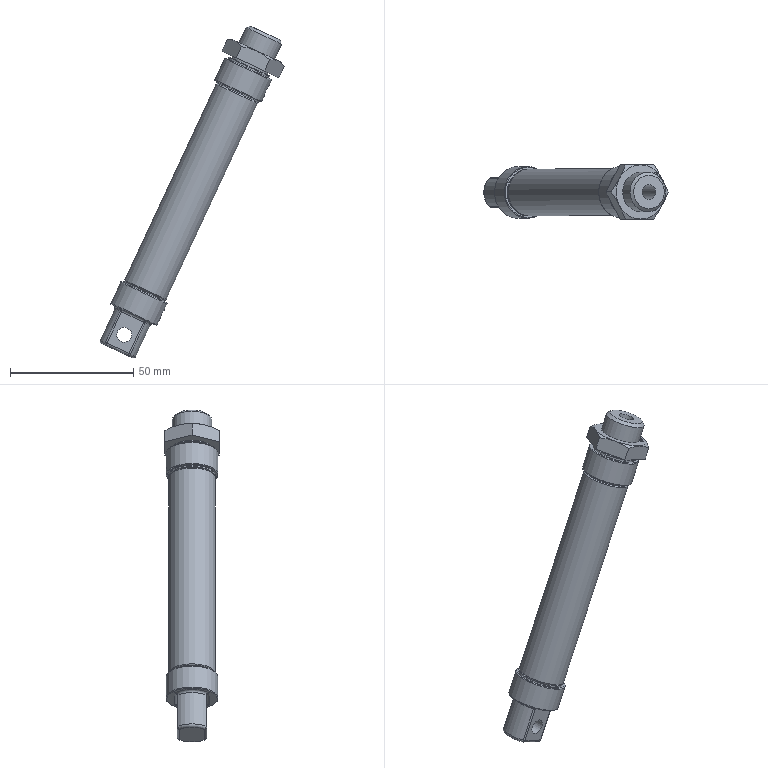Part | STEP file | 冲床-300配套压波_id666_x_t | 1 solid | 138 faces | box 74.68 x 22 x 134.608 mm | volume 35462 mm3 | plane 67 | cylinder 45 | cone 10 | torus 8 | spline 4 | sphere 4 | commonest cylinder face diameters 2 x8 1.006 x4 1.247 x4 16 x4 1.749 x3 18.9 x3